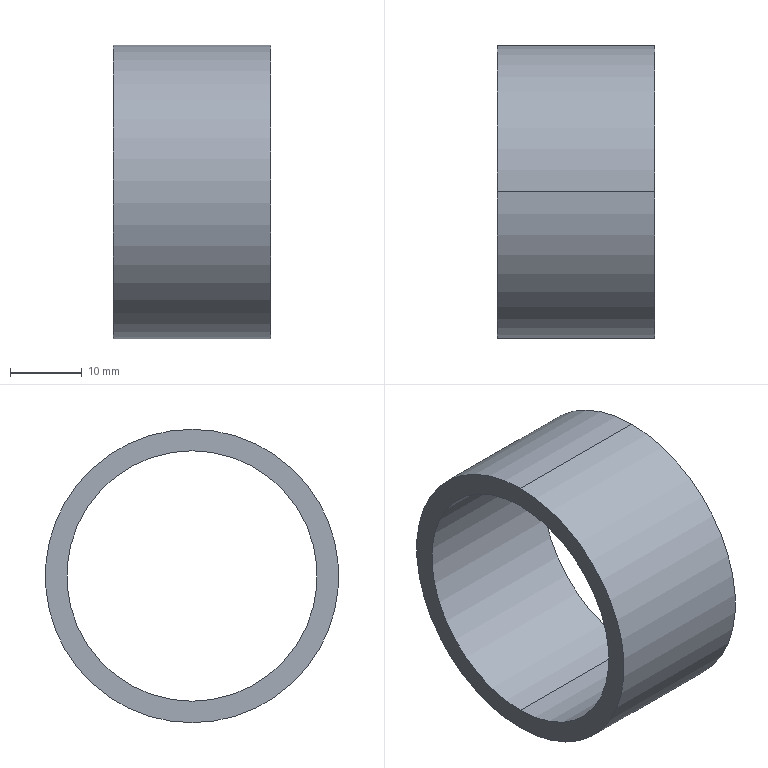Part | SolidWorks | features Extrusion 1 | 1 solid | 6 faces | box 22 x 41 x 41 mm | volume 7879 mm3 | cylinder 4 | plane 2 | commonest cylinder face diameters 35 x2 41 x2
STEP:
#1=CARTESIAN_POINT('',(22.,0.,17.5));
#2=VERTEX_POINT('',#1);
#3=CARTESIAN_POINT('',(22.,0.,-17.5));
#4=VERTEX_POINT('',#3);
#5=CARTESIAN_POINT('',(22.,0.,0.));
#6=DIRECTION('',(1.,0.,0.));
#7=DIRECTION('',(0.,0.,-1.));
#8=AXIS2_PLACEMENT_3D('',#5,#6,#7);
#9=CIRCLE('',#8,17.5);
#10=EDGE_CURVE('',#2,#4,#9,.T.);
#11=ORIENTED_EDGE('',*,*,#10,.T.);
#12=CARTESIAN_POINT('',(0.,0.,-17.5));
#13=VERTEX_POINT('',#12);
#14=CARTESIAN_POINT('',(22.,0.,-17.5));
#15=DIRECTION('',(-1.,0.,0.));
#16=VECTOR('',#15,1000.);
#17=LINE('',#14,#16);
#18=EDGE_CURVE('',#4,#13,#17,.T.);
#19=ORIENTED_EDGE('',*,*,#18,.T.);
#20=CARTESIAN_POINT('',(0.,0.,17.5));
#21=VERTEX_POINT('',#20);
#22=CARTESIAN_POINT('',(0.,0.,0.));
#23=DIRECTION('',(1.,0.,0.));
#24=DIRECTION('',(0.,0.,-1.));
#25=AXIS2_PLACEMENT_3D('',#22,#23,#24);
#26=CIRCLE('',#25,17.5);
#27=EDGE_CURVE('',#21,#13,#26,.T.);
#28=ORIENTED_EDGE('',*,*,#27,.F.);
#29=CARTESIAN_POINT('',(22.,0.,17.5));
#30=DIRECTION('',(-1.,0.,0.));
#31=VECTOR('',#30,1000.);
#32=LINE('',#29,#31);
#33=EDGE_CURVE('',#2,#21,#32,.T.);
#34=ORIENTED_EDGE('',*,*,#33,.F.);
#35=EDGE_LOOP('',(#11,#19,#28,#34));
#36=FACE_OUTER_BOUND('',#35,.T.);
#37=CARTESIAN_POINT('',(22.,0.,0.));
#38=DIRECTION('',(-1.,0.,0.));
#39=DIRECTION('',(0.,0.,1.));
#40=AXIS2_PLACEMENT_3D('',#37,#38,#39);
#41=CYLINDRICAL_SURFACE('',#40,17.5);
#42=ADVANCED_FACE('',(#36),#41,.F.);
#43=CARTESIAN_POINT('',(22.,0.,-20.5));
#44=VERTEX_POINT('',#43);
#45=CARTESIAN_POINT('',(22.,0.,20.5));
#46=VERTEX_POINT('',#45);
#47=CARTESIAN_POINT('',(22.,0.,0.));
#48=DIRECTION('',(1.,0.,0.));
#49=DIRECTION('',(0.,0.,-1.));
#50=AXIS2_PLACEMENT_3D('',#47,#48,#49);
#51=CIRCLE('',#50,20.5);
#52=EDGE_CURVE('',#44,#46,#51,.T.);
#53=ORIENTED_EDGE('',*,*,#52,.F.);
#54=CARTESIAN_POINT('',(0.,0.,-20.5));
#55=VERTEX_POINT('',#54);
#56=CARTESIAN_POINT('',(22.,0.,-20.5));
#57=DIRECTION('',(-1.,0.,0.));
#58=VECTOR('',#57,1000.);
#59=LINE('',#56,#58);
#60=EDGE_CURVE('',#44,#55,#59,.T.);
#61=ORIENTED_EDGE('',*,*,#60,.T.);
#62=CARTESIAN_POINT('',(0.,0.,20.5));
#63=VERTEX_POINT('',#62);
#64=CARTESIAN_POINT('',(0.,0.,0.));
#65=DIRECTION('',(1.,0.,0.));
#66=DIRECTION('',(0.,0.,-1.));
#67=AXIS2_PLACEMENT_3D('',#64,#65,#66);
#68=CIRCLE('',#67,20.5);
#69=EDGE_CURVE('',#55,#63,#68,.T.);
#70=ORIENTED_EDGE('',*,*,#69,.T.);
#71=CARTESIAN_POINT('',(22.,0.,20.5));
#72=DIRECTION('',(-1.,0.,0.));
#73=VECTOR('',#72,1000.);
#74=LINE('',#71,#73);
#75=EDGE_CURVE('',#46,#63,#74,.T.);
#76=ORIENTED_EDGE('',*,*,#75,.F.);
#77=EDGE_LOOP('',(#53,#61,#70,#76));
#78=FACE_OUTER_BOUND('',#77,.T.);
#79=CARTESIAN_POINT('',(22.,0.,0.));
#80=DIRECTION('',(-1.,0.,0.));
#81=DIRECTION('',(0.,0.,1.));
#82=AXIS2_PLACEMENT_3D('',#79,#80,#81);
#83=CYLINDRICAL_SURFACE('',#82,20.5);
#84=ADVANCED_FACE('',(#78),#83,.T.);
#85=CARTESIAN_POINT('',(22.,0.,0.));
#86=DIRECTION('',(1.,0.,0.));
#87=DIRECTION('',(0.,0.,-1.));
#88=AXIS2_PLACEMENT_3D('',#85,#86,#87);
#89=CIRCLE('',#88,20.5);
#90=EDGE_CURVE('',#46,#44,#89,.T.);
#91=ORIENTED_EDGE('',*,*,#90,.T.);
#92=ORIENTED_EDGE('',*,*,#52,.T.);
#93=EDGE_LOOP('',(#91,#92));
#94=FACE_OUTER_BOUND('',#93,.T.);
#95=ORIENTED_EDGE('',*,*,#10,.F.);
#96=CARTESIAN_POINT('',(22.,0.,0.));
#97=DIRECTION('',(1.,0.,0.));
#98=DIRECTION('',(0.,0.,-1.));
#99=AXIS2_PLACEMENT_3D('',#96,#97,#98);
#100=CIRCLE('',#99,17.5);
#101=EDGE_CURVE('',#4,#2,#100,.T.);
#102=ORIENTED_EDGE('',*,*,#101,.F.);
#103=EDGE_LOOP('',(#95,#102));
#104=FACE_BOUND('',#103,.T.);
#105=CARTESIAN_POINT('',(22.,0.,0.));
#106=DIRECTION('',(1.,0.,0.));
#107=DIRECTION('',(0.,0.,-1.));
#108=AXIS2_PLACEMENT_3D('',#105,#106,#107);
#109=PLANE('',#108);
#110=ADVANCED_FACE('',(#94,#104),#109,.T.);
#111=CARTESIAN_POINT('',(0.,0.,0.));
#112=DIRECTION('',(1.,0.,0.));
#113=DIRECTION('',(0.,0.,-1.));
#114=AXIS2_PLACEMENT_3D('',#111,#112,#113);
#115=CIRCLE('',#114,20.5);
#116=EDGE_CURVE('',#63,#55,#115,.T.);
#117=ORIENTED_EDGE('',*,*,#116,.F.);
#118=ORIENTED_EDGE('',*,*,#69,.F.);
#119=EDGE_LOOP('',(#117,#118));
#120=FACE_OUTER_BOUND('',#119,.T.);
#121=ORIENTED_EDGE('',*,*,#27,.T.);
#122=CARTESIAN_POINT('',(0.,0.,0.));
#123=DIRECTION('',(1.,0.,0.));
#124=DIRECTION('',(0.,0.,-1.));
#125=AXIS2_PLACEMENT_3D('',#122,#123,#124);
#126=CIRCLE('',#125,17.5);
#127=EDGE_CURVE('',#13,#21,#126,.T.);
#128=ORIENTED_EDGE('',*,*,#127,.T.);
#129=EDGE_LOOP('',(#121,#128));
#130=FACE_BOUND('',#129,.T.);
#131=CARTESIAN_POINT('',(0.,0.,0.));
#132=DIRECTION('',(1.,0.,0.));
#133=DIRECTION('',(0.,0.,-1.));
#134=AXIS2_PLACEMENT_3D('',#131,#132,#133);
#135=PLANE('',#134);
#136=ADVANCED_FACE('',(#120,#130),#135,.F.);
#137=ORIENTED_EDGE('',*,*,#60,.F.);
#138=ORIENTED_EDGE('',*,*,#90,.F.);
#139=ORIENTED_EDGE('',*,*,#75,.T.);
#140=ORIENTED_EDGE('',*,*,#116,.T.);
#141=EDGE_LOOP('',(#137,#138,#139,#140));
#142=FACE_OUTER_BOUND('',#141,.T.);
#143=CARTESIAN_POINT('',(22.,0.,0.));
#144=DIRECTION('',(-1.,0.,0.));
#145=DIRECTION('',(0.,0.,1.));
#146=AXIS2_PLACEMENT_3D('',#143,#144,#145);
#147=CYLINDRICAL_SURFACE('',#146,20.5);
#148=ADVANCED_FACE('',(#142),#147,.T.);
#149=ORIENTED_EDGE('',*,*,#18,.F.);
#150=ORIENTED_EDGE('',*,*,#101,.T.);
#151=ORIENTED_EDGE('',*,*,#33,.T.);
#152=ORIENTED_EDGE('',*,*,#127,.F.);
#153=EDGE_LOOP('',(#149,#150,#151,#152));
#154=FACE_OUTER_BOUND('',#153,.T.);
#155=CARTESIAN_POINT('',(22.,0.,0.));
#156=DIRECTION('',(-1.,0.,0.));
#157=DIRECTION('',(0.,0.,1.));
#158=AXIS2_PLACEMENT_3D('',#155,#156,#157);
#159=CYLINDRICAL_SURFACE('',#158,17.5);
#160=ADVANCED_FACE('',(#154),#159,.F.);
#161=CLOSED_SHELL('',(#42,#84,#110,#136,#148,#160));
#162=MANIFOLD_SOLID_BREP('',#161);
#163=CARTESIAN_POINT('',(0.,0.,0.));
#164=DIRECTION('',(0.,0.,1.));
#165=DIRECTION('',(1.,0.,0.));
#166=AXIS2_PLACEMENT_3D('',#163,#164,#165);
#167=(LENGTH_UNIT()NAMED_UNIT(*)SI_UNIT(.MILLI.,.METRE.));
#168=UNCERTAINTY_MEASURE_WITH_UNIT(LENGTH_MEASURE(0.00001),#167,'','');
#169=(NAMED_UNIT(*)PLANE_ANGLE_UNIT()SI_UNIT($,.RADIAN.));
#170=(NAMED_UNIT(*)SI_UNIT($,.STERADIAN.)SOLID_ANGLE_UNIT());
#171=(GEOMETRIC_REPRESENTATION_CONTEXT(3)GLOBAL_UNCERTAINTY_ASSIGNED_CONTEXT((#168))GLOBAL_UNIT_ASSIGNED_CONTEXT((#167,#169,#170))REPRESENTATION_CONTEXT('',''));
#172=ADVANCED_BREP_SHAPE_REPRESENTATION('',(#162,#166),#171);